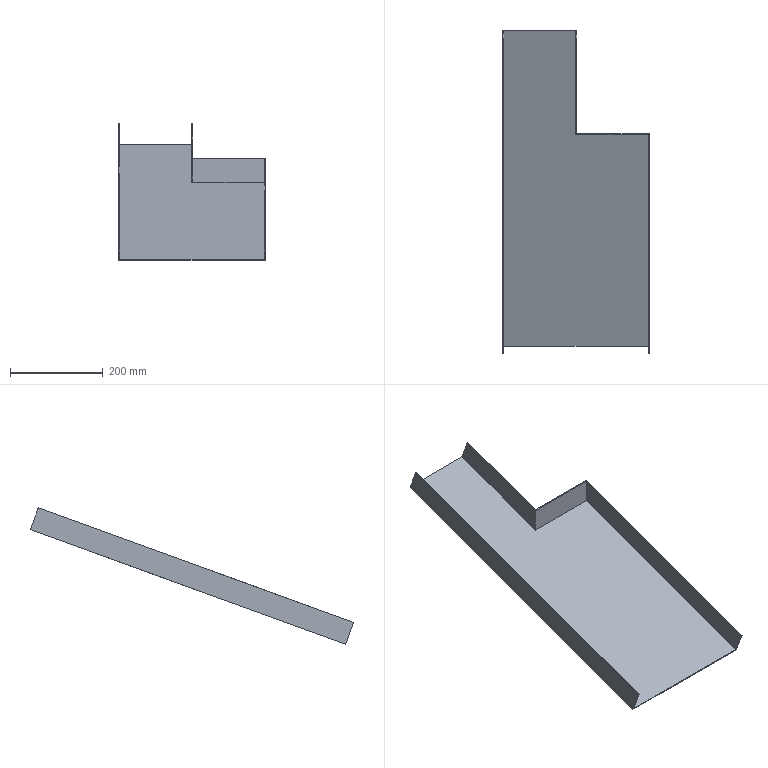Part | NX | features solid 2 | 1 solid | 14 faces | box 315 x 695.354 x 293.848 mm | volume 535547 mm3 | plane 14
STEP:
#1=CARTESIAN_POINT('',(-807.,-517.,-239.51));
#2=VERTEX_POINT('',#1);
#3=CARTESIAN_POINT('',(-963.,-517.,-239.51));
#4=VERTEX_POINT('',#3);
#5=CARTESIAN_POINT('',(-1225.,-517.,-239.51));
#6=DIRECTION('',(1.,0.,0.));
#7=VECTOR('',#6,1000.);
#8=LINE('',#5,#7);
#9=EDGE_CURVE('',#2,#4,#8,.F.);
#10=ORIENTED_EDGE('',*,*,#9,.T.);
#11=CARTESIAN_POINT('',(-963.,-293.385,-158.121));
#12=VERTEX_POINT('',#11);
#13=CARTESIAN_POINT('',(-963.,108.795,-11.739));
#14=DIRECTION('',(0.,0.9397,0.342));
#15=VECTOR('',#14,1000.);
#16=LINE('',#13,#15);
#17=EDGE_CURVE('',#4,#12,#16,.T.);
#18=ORIENTED_EDGE('',*,*,#17,.T.);
#19=CARTESIAN_POINT('',(-1118.,-293.385,-158.121));
#20=VERTEX_POINT('',#19);
#21=CARTESIAN_POINT('',(-1225.,-293.385,-158.121));
#22=DIRECTION('',(-1.,0.,0.));
#23=VECTOR('',#22,1000.);
#24=LINE('',#21,#23);
#25=EDGE_CURVE('',#20,#12,#24,.F.);
#26=ORIENTED_EDGE('',*,*,#25,.F.);
#27=CARTESIAN_POINT('',(-1118.,-971.638,-404.984));
#28=VERTEX_POINT('',#27);
#29=CARTESIAN_POINT('',(-1118.,108.795,-11.739));
#30=DIRECTION('',(0.,-0.9397,-0.342));
#31=VECTOR('',#30,1000.);
#32=LINE('',#29,#31);
#33=EDGE_CURVE('',#20,#28,#32,.T.);
#34=ORIENTED_EDGE('',*,*,#33,.T.);
#35=CARTESIAN_POINT('',(-807.,-971.638,-404.984));
#36=VERTEX_POINT('',#35);
#37=CARTESIAN_POINT('',(-1100.,-971.638,-404.984));
#38=DIRECTION('',(1.,0.,0.));
#39=VECTOR('',#38,1000.);
#40=LINE('',#37,#39);
#41=EDGE_CURVE('',#28,#36,#40,.T.);
#42=ORIENTED_EDGE('',*,*,#41,.T.);
#43=CARTESIAN_POINT('',(-807.,-515.684,-239.031));
#44=DIRECTION('',(0.,-0.9397,-0.342));
#45=VECTOR('',#44,1000.);
#46=LINE('',#43,#45);
#47=EDGE_CURVE('',#2,#36,#46,.T.);
#48=ORIENTED_EDGE('',*,*,#47,.F.);
#49=EDGE_LOOP('',(#10,#18,#26,#34,#42,#48));
#50=FACE_BOUND('',#49,.T.);
#51=CARTESIAN_POINT('',(-1225.,108.795,-11.739));
#52=DIRECTION('',(0.,0.342,-0.9397));
#53=DIRECTION('',(0.,-0.9397,-0.342));
#54=AXIS2_PLACEMENT_3D('',#51,#52,#53);
#55=PLANE('',#54);
#56=ADVANCED_FACE('',(#50),#55,.F.);
#57=CARTESIAN_POINT('',(-961.,-515.,-240.91));
#58=VERTEX_POINT('',#57);
#59=CARTESIAN_POINT('',(-961.,-515.,-187.701));
#60=VERTEX_POINT('',#59);
#61=CARTESIAN_POINT('',(-961.,-515.,-240.91));
#62=DIRECTION('',(0.,0.,-1.));
#63=VECTOR('',#62,1000.);
#64=LINE('',#61,#63);
#65=EDGE_CURVE('',#58,#60,#64,.F.);
#66=ORIENTED_EDGE('',*,*,#65,.F.);
#67=CARTESIAN_POINT('',(-961.,-292.701,-160.));
#68=VERTEX_POINT('',#67);
#69=CARTESIAN_POINT('',(-961.,109.479,-13.618));
#70=DIRECTION('',(0.,0.9397,0.342));
#71=VECTOR('',#70,1000.);
#72=LINE('',#69,#71);
#73=EDGE_CURVE('',#58,#68,#72,.T.);
#74=ORIENTED_EDGE('',*,*,#73,.T.);
#75=CARTESIAN_POINT('',(-961.,-309.802,-113.015));
#76=VERTEX_POINT('',#75);
#77=CARTESIAN_POINT('',(-961.,-292.701,-160.));
#78=DIRECTION('',(0.,-0.342,0.9397));
#79=VECTOR('',#78,1000.);
#80=LINE('',#77,#79);
#81=EDGE_CURVE('',#68,#76,#80,.T.);
#82=ORIENTED_EDGE('',*,*,#81,.T.);
#83=CARTESIAN_POINT('',(-961.,-532.101,-193.926));
#84=DIRECTION('',(0.,0.9397,0.342));
#85=VECTOR('',#84,1000.);
#86=LINE('',#83,#85);
#87=EDGE_CURVE('',#60,#76,#86,.T.);
#88=ORIENTED_EDGE('',*,*,#87,.F.);
#89=EDGE_LOOP('',(#66,#74,#82,#88));
#90=FACE_BOUND('',#89,.T.);
#91=CARTESIAN_POINT('',(-961.,109.479,-13.618));
#92=DIRECTION('',(-1.,0.,0.));
#93=DIRECTION('',(0.,0.,1.));
#94=AXIS2_PLACEMENT_3D('',#91,#92,#93);
#95=PLANE('',#94);
#96=ADVANCED_FACE('',(#90),#95,.F.);
#97=ORIENTED_EDGE('',*,*,#47,.T.);
#98=CARTESIAN_POINT('',(-807.,-988.055,-359.879));
#99=VERTEX_POINT('',#98);
#100=CARTESIAN_POINT('',(-807.,-988.055,-359.879));
#101=DIRECTION('',(0.,0.342,-0.9397));
#102=VECTOR('',#101,1000.);
#103=LINE('',#100,#102);
#104=EDGE_CURVE('',#99,#36,#103,.T.);
#105=ORIENTED_EDGE('',*,*,#104,.F.);
#106=CARTESIAN_POINT('',(-807.,-517.,-188.429));
#107=VERTEX_POINT('',#106);
#108=CARTESIAN_POINT('',(-807.,-532.101,-193.926));
#109=DIRECTION('',(0.,0.9397,0.342));
#110=VECTOR('',#109,1000.);
#111=LINE('',#108,#110);
#112=EDGE_CURVE('',#107,#99,#111,.F.);
#113=ORIENTED_EDGE('',*,*,#112,.F.);
#114=CARTESIAN_POINT('',(-807.,-517.,-240.91));
#115=DIRECTION('',(0.,0.,-1.));
#116=VECTOR('',#115,1000.);
#117=LINE('',#114,#116);
#118=EDGE_CURVE('',#2,#107,#117,.F.);
#119=ORIENTED_EDGE('',*,*,#118,.F.);
#120=EDGE_LOOP('',(#97,#105,#113,#119));
#121=FACE_BOUND('',#120,.T.);
#122=CARTESIAN_POINT('',(-807.,-532.101,-193.926));
#123=DIRECTION('',(-1.,0.,0.));
#124=DIRECTION('',(0.,0.,1.));
#125=AXIS2_PLACEMENT_3D('',#122,#123,#124);
#126=PLANE('',#125);
#127=ADVANCED_FACE('',(#121),#126,.T.);
#128=CARTESIAN_POINT('',(-1120.,-970.954,-406.864));
#129=VERTEX_POINT('',#128);
#130=CARTESIAN_POINT('',(-1120.,-988.055,-359.879));
#131=VERTEX_POINT('',#130);
#132=CARTESIAN_POINT('',(-1120.,-970.954,-406.864));
#133=DIRECTION('',(0.,-0.342,0.9397));
#134=VECTOR('',#133,1000.);
#135=LINE('',#132,#134);
#136=EDGE_CURVE('',#129,#131,#135,.T.);
#137=ORIENTED_EDGE('',*,*,#136,.F.);
#138=CARTESIAN_POINT('',(-805.,-970.954,-406.864));
#139=VERTEX_POINT('',#138);
#140=CARTESIAN_POINT('',(-1100.,-970.954,-406.864));
#141=DIRECTION('',(1.,0.,0.));
#142=VECTOR('',#141,1000.);
#143=LINE('',#140,#142);
#144=EDGE_CURVE('',#129,#139,#143,.T.);
#145=ORIENTED_EDGE('',*,*,#144,.T.);
#146=CARTESIAN_POINT('',(-805.,-988.055,-359.879));
#147=VERTEX_POINT('',#146);
#148=CARTESIAN_POINT('',(-805.,-970.954,-406.864));
#149=DIRECTION('',(0.,-0.342,0.9397));
#150=VECTOR('',#149,1000.);
#151=LINE('',#148,#150);
#152=EDGE_CURVE('',#139,#147,#151,.T.);
#153=ORIENTED_EDGE('',*,*,#152,.T.);
#154=CARTESIAN_POINT('',(-870.,-988.055,-359.879));
#155=DIRECTION('',(1.,0.,0.));
#156=VECTOR('',#155,1000.);
#157=LINE('',#154,#156);
#158=EDGE_CURVE('',#147,#99,#157,.F.);
#159=ORIENTED_EDGE('',*,*,#158,.T.);
#160=ORIENTED_EDGE('',*,*,#104,.T.);
#161=ORIENTED_EDGE('',*,*,#41,.F.);
#162=CARTESIAN_POINT('',(-1118.,-988.055,-359.879));
#163=VERTEX_POINT('',#162);
#164=CARTESIAN_POINT('',(-1118.,-988.055,-359.879));
#165=DIRECTION('',(0.,0.342,-0.9397));
#166=VECTOR('',#165,1000.);
#167=LINE('',#164,#166);
#168=EDGE_CURVE('',#163,#28,#167,.T.);
#169=ORIENTED_EDGE('',*,*,#168,.F.);
#170=CARTESIAN_POINT('',(-1120.,-988.055,-359.879));
#171=DIRECTION('',(1.,0.,0.));
#172=VECTOR('',#171,1000.);
#173=LINE('',#170,#172);
#174=EDGE_CURVE('',#131,#163,#173,.T.);
#175=ORIENTED_EDGE('',*,*,#174,.F.);
#176=EDGE_LOOP('',(#137,#145,#153,#159,#160,#161,#169,#175));
#177=FACE_BOUND('',#176,.T.);
#178=CARTESIAN_POINT('',(-1100.,-970.954,-406.864));
#179=DIRECTION('',(0.,0.9397,0.342));
#180=DIRECTION('',(0.,0.342,-0.9397));
#181=AXIS2_PLACEMENT_3D('',#178,#179,#180);
#182=PLANE('',#181);
#183=ADVANCED_FACE('',(#177),#182,.F.);
#184=CARTESIAN_POINT('',(-1120.,-292.701,-160.));
#185=VERTEX_POINT('',#184);
#186=CARTESIAN_POINT('',(-1120.,-309.802,-113.015));
#187=VERTEX_POINT('',#186);
#188=CARTESIAN_POINT('',(-1120.,-292.701,-160.));
#189=DIRECTION('',(0.,-0.342,0.9397));
#190=VECTOR('',#189,1000.);
#191=LINE('',#188,#190);
#192=EDGE_CURVE('',#185,#187,#191,.T.);
#193=ORIENTED_EDGE('',*,*,#192,.F.);
#194=CARTESIAN_POINT('',(-1120.,109.479,-13.618));
#195=DIRECTION('',(0.,0.9397,0.342));
#196=VECTOR('',#195,1000.);
#197=LINE('',#194,#196);
#198=EDGE_CURVE('',#185,#129,#197,.F.);
#199=ORIENTED_EDGE('',*,*,#198,.T.);
#200=ORIENTED_EDGE('',*,*,#136,.T.);
#201=CARTESIAN_POINT('',(-1120.,-309.802,-113.015));
#202=DIRECTION('',(0.,-0.9397,-0.342));
#203=VECTOR('',#202,1000.);
#204=LINE('',#201,#203);
#205=EDGE_CURVE('',#187,#131,#204,.T.);
#206=ORIENTED_EDGE('',*,*,#205,.F.);
#207=EDGE_LOOP('',(#193,#199,#200,#206));
#208=FACE_BOUND('',#207,.T.);
#209=CARTESIAN_POINT('',(-1120.,109.479,-13.618));
#210=DIRECTION('',(1.,0.,0.));
#211=DIRECTION('',(0.,0.,-1.));
#212=AXIS2_PLACEMENT_3D('',#209,#210,#211);
#213=PLANE('',#212);
#214=ADVANCED_FACE('',(#208),#213,.F.);
#215=CARTESIAN_POINT('',(-1225.,-292.701,-160.));
#216=DIRECTION('',(-1.,0.,0.));
#217=VECTOR('',#216,1000.);
#218=LINE('',#215,#217);
#219=EDGE_CURVE('',#185,#68,#218,.F.);
#220=ORIENTED_EDGE('',*,*,#219,.F.);
#221=ORIENTED_EDGE('',*,*,#192,.T.);
#222=CARTESIAN_POINT('',(-1118.,-309.802,-113.015));
#223=VERTEX_POINT('',#222);
#224=CARTESIAN_POINT('',(-1120.,-309.802,-113.015));
#225=DIRECTION('',(1.,0.,0.));
#226=VECTOR('',#225,1000.);
#227=LINE('',#224,#226);
#228=EDGE_CURVE('',#187,#223,#227,.T.);
#229=ORIENTED_EDGE('',*,*,#228,.T.);
#230=CARTESIAN_POINT('',(-1118.,-309.802,-113.015));
#231=DIRECTION('',(0.,0.342,-0.9397));
#232=VECTOR('',#231,1000.);
#233=LINE('',#230,#232);
#234=EDGE_CURVE('',#223,#20,#233,.T.);
#235=ORIENTED_EDGE('',*,*,#234,.T.);
#236=ORIENTED_EDGE('',*,*,#25,.T.);
#237=CARTESIAN_POINT('',(-963.,-309.802,-113.015));
#238=VERTEX_POINT('',#237);
#239=CARTESIAN_POINT('',(-963.,-309.802,-113.015));
#240=DIRECTION('',(0.,0.342,-0.9397));
#241=VECTOR('',#240,1000.);
#242=LINE('',#239,#241);
#243=EDGE_CURVE('',#238,#12,#242,.T.);
#244=ORIENTED_EDGE('',*,*,#243,.F.);
#245=CARTESIAN_POINT('',(-961.,-309.802,-113.015));
#246=DIRECTION('',(1.,0.,0.));
#247=VECTOR('',#246,1000.);
#248=LINE('',#245,#247);
#249=EDGE_CURVE('',#76,#238,#248,.F.);
#250=ORIENTED_EDGE('',*,*,#249,.F.);
#251=ORIENTED_EDGE('',*,*,#81,.F.);
#252=EDGE_LOOP('',(#220,#221,#229,#235,#236,#244,#250,#251));
#253=FACE_BOUND('',#252,.T.);
#254=CARTESIAN_POINT('',(-1225.,-292.701,-160.));
#255=DIRECTION('',(0.,0.9397,0.342));
#256=DIRECTION('',(0.,0.342,-0.9397));
#257=AXIS2_PLACEMENT_3D('',#254,#255,#256);
#258=PLANE('',#257);
#259=ADVANCED_FACE('',(#253),#258,.T.);
#260=CARTESIAN_POINT('',(-805.,-515.,-187.701));
#261=VERTEX_POINT('',#260);
#262=CARTESIAN_POINT('',(-805.,-532.101,-193.926));
#263=DIRECTION('',(0.,0.9397,0.342));
#264=VECTOR('',#263,1000.);
#265=LINE('',#262,#264);
#266=EDGE_CURVE('',#261,#147,#265,.F.);
#267=ORIENTED_EDGE('',*,*,#266,.T.);
#268=ORIENTED_EDGE('',*,*,#152,.F.);
#269=CARTESIAN_POINT('',(-805.,-515.,-240.91));
#270=VERTEX_POINT('',#269);
#271=CARTESIAN_POINT('',(-805.,109.479,-13.618));
#272=DIRECTION('',(0.,-0.9397,-0.342));
#273=VECTOR('',#272,1000.);
#274=LINE('',#271,#273);
#275=EDGE_CURVE('',#270,#139,#274,.T.);
#276=ORIENTED_EDGE('',*,*,#275,.F.);
#277=CARTESIAN_POINT('',(-805.,-515.,-240.91));
#278=DIRECTION('',(0.,0.,1.));
#279=VECTOR('',#278,1000.);
#280=LINE('',#277,#279);
#281=EDGE_CURVE('',#270,#261,#280,.T.);
#282=ORIENTED_EDGE('',*,*,#281,.T.);
#283=EDGE_LOOP('',(#267,#268,#276,#282));
#284=FACE_BOUND('',#283,.T.);
#285=CARTESIAN_POINT('',(-805.,109.479,-13.618));
#286=DIRECTION('',(1.,0.,0.));
#287=DIRECTION('',(0.,0.,-1.));
#288=AXIS2_PLACEMENT_3D('',#285,#286,#287);
#289=PLANE('',#288);
#290=ADVANCED_FACE('',(#284),#289,.T.);
#291=ORIENTED_EDGE('',*,*,#144,.F.);
#292=ORIENTED_EDGE('',*,*,#198,.F.);
#293=ORIENTED_EDGE('',*,*,#219,.T.);
#294=ORIENTED_EDGE('',*,*,#73,.F.);
#295=CARTESIAN_POINT('',(-1225.,-515.,-240.91));
#296=DIRECTION('',(-1.,0.,0.));
#297=VECTOR('',#296,1000.);
#298=LINE('',#295,#297);
#299=EDGE_CURVE('',#270,#58,#298,.T.);
#300=ORIENTED_EDGE('',*,*,#299,.F.);
#301=ORIENTED_EDGE('',*,*,#275,.T.);
#302=EDGE_LOOP('',(#291,#292,#293,#294,#300,#301));
#303=FACE_BOUND('',#302,.T.);
#304=CARTESIAN_POINT('',(-1225.,109.479,-13.618));
#305=DIRECTION('',(0.,0.342,-0.9397));
#306=DIRECTION('',(0.,-0.9397,-0.342));
#307=AXIS2_PLACEMENT_3D('',#304,#305,#306);
#308=PLANE('',#307);
#309=ADVANCED_FACE('',(#303),#308,.T.);
#310=CARTESIAN_POINT('',(-963.,-517.,-188.429));
#311=VERTEX_POINT('',#310);
#312=CARTESIAN_POINT('',(-961.,-517.,-188.429));
#313=DIRECTION('',(-1.,0.,0.));
#314=VECTOR('',#313,1000.);
#315=LINE('',#312,#314);
#316=EDGE_CURVE('',#107,#311,#315,.T.);
#317=ORIENTED_EDGE('',*,*,#316,.T.);
#318=CARTESIAN_POINT('',(-963.,-517.,-193.926));
#319=DIRECTION('',(0.,0.,1.));
#320=VECTOR('',#319,1000.);
#321=LINE('',#318,#320);
#322=EDGE_CURVE('',#311,#4,#321,.F.);
#323=ORIENTED_EDGE('',*,*,#322,.T.);
#324=ORIENTED_EDGE('',*,*,#9,.F.);
#325=ORIENTED_EDGE('',*,*,#118,.T.);
#326=EDGE_LOOP('',(#317,#323,#324,#325));
#327=FACE_BOUND('',#326,.T.);
#328=CARTESIAN_POINT('',(-870.,-517.,-240.91));
#329=DIRECTION('',(0.,-1.,0.));
#330=DIRECTION('',(-1.,0.,0.));
#331=AXIS2_PLACEMENT_3D('',#328,#329,#330);
#332=PLANE('',#331);
#333=ADVANCED_FACE('',(#327),#332,.T.);
#334=ORIENTED_EDGE('',*,*,#322,.F.);
#335=CARTESIAN_POINT('',(-963.,-532.101,-193.926));
#336=DIRECTION('',(0.,0.9397,0.342));
#337=VECTOR('',#336,1000.);
#338=LINE('',#335,#337);
#339=EDGE_CURVE('',#311,#238,#338,.T.);
#340=ORIENTED_EDGE('',*,*,#339,.T.);
#341=ORIENTED_EDGE('',*,*,#243,.T.);
#342=ORIENTED_EDGE('',*,*,#17,.F.);
#343=EDGE_LOOP('',(#334,#340,#341,#342));
#344=FACE_BOUND('',#343,.T.);
#345=CARTESIAN_POINT('',(-963.,-532.101,-193.926));
#346=DIRECTION('',(1.,0.,0.));
#347=DIRECTION('',(0.,0.,-1.));
#348=AXIS2_PLACEMENT_3D('',#345,#346,#347);
#349=PLANE('',#348);
#350=ADVANCED_FACE('',(#344),#349,.F.);
#351=ORIENTED_EDGE('',*,*,#316,.F.);
#352=ORIENTED_EDGE('',*,*,#112,.T.);
#353=ORIENTED_EDGE('',*,*,#158,.F.);
#354=ORIENTED_EDGE('',*,*,#266,.F.);
#355=CARTESIAN_POINT('',(-870.,-515.,-187.701));
#356=DIRECTION('',(-1.,0.,0.));
#357=VECTOR('',#356,1000.);
#358=LINE('',#355,#357);
#359=EDGE_CURVE('',#261,#60,#358,.T.);
#360=ORIENTED_EDGE('',*,*,#359,.T.);
#361=ORIENTED_EDGE('',*,*,#87,.T.);
#362=ORIENTED_EDGE('',*,*,#249,.T.);
#363=ORIENTED_EDGE('',*,*,#339,.F.);
#364=EDGE_LOOP('',(#351,#352,#353,#354,#360,#361,#362,#363));
#365=FACE_BOUND('',#364,.T.);
#366=CARTESIAN_POINT('',(-961.,-532.101,-193.926));
#367=DIRECTION('',(0.,-0.342,0.9397));
#368=DIRECTION('',(0.,0.9397,0.342));
#369=AXIS2_PLACEMENT_3D('',#366,#367,#368);
#370=PLANE('',#369);
#371=ADVANCED_FACE('',(#365),#370,.T.);
#372=ORIENTED_EDGE('',*,*,#234,.F.);
#373=CARTESIAN_POINT('',(-1118.,-309.802,-113.015));
#374=DIRECTION('',(0.,-0.9397,-0.342));
#375=VECTOR('',#374,1000.);
#376=LINE('',#373,#375);
#377=EDGE_CURVE('',#223,#163,#376,.T.);
#378=ORIENTED_EDGE('',*,*,#377,.T.);
#379=ORIENTED_EDGE('',*,*,#168,.T.);
#380=ORIENTED_EDGE('',*,*,#33,.F.);
#381=EDGE_LOOP('',(#372,#378,#379,#380));
#382=FACE_BOUND('',#381,.T.);
#383=CARTESIAN_POINT('',(-1118.,-309.802,-113.015));
#384=DIRECTION('',(-1.,0.,0.));
#385=DIRECTION('',(0.,0.,1.));
#386=AXIS2_PLACEMENT_3D('',#383,#384,#385);
#387=PLANE('',#386);
#388=ADVANCED_FACE('',(#382),#387,.F.);
#389=ORIENTED_EDGE('',*,*,#174,.T.);
#390=ORIENTED_EDGE('',*,*,#377,.F.);
#391=ORIENTED_EDGE('',*,*,#228,.F.);
#392=ORIENTED_EDGE('',*,*,#205,.T.);
#393=EDGE_LOOP('',(#389,#390,#391,#392));
#394=FACE_BOUND('',#393,.T.);
#395=CARTESIAN_POINT('',(-1120.,-309.802,-113.015));
#396=DIRECTION('',(0.,-0.342,0.9397));
#397=DIRECTION('',(0.,-0.9397,-0.342));
#398=AXIS2_PLACEMENT_3D('',#395,#396,#397);
#399=PLANE('',#398);
#400=ADVANCED_FACE('',(#394),#399,.T.);
#401=ORIENTED_EDGE('',*,*,#281,.F.);
#402=ORIENTED_EDGE('',*,*,#299,.T.);
#403=ORIENTED_EDGE('',*,*,#65,.T.);
#404=ORIENTED_EDGE('',*,*,#359,.F.);
#405=EDGE_LOOP('',(#401,#402,#403,#404));
#406=FACE_BOUND('',#405,.T.);
#407=CARTESIAN_POINT('',(-870.,-515.,-240.91));
#408=DIRECTION('',(0.,-1.,0.));
#409=DIRECTION('',(-1.,0.,0.));
#410=AXIS2_PLACEMENT_3D('',#407,#408,#409);
#411=PLANE('',#410);
#412=ADVANCED_FACE('',(#406),#411,.F.);
#413=CLOSED_SHELL('',(#56,#96,#127,#183,#214,#259,#290,#309,#333,#350,#371,#388,#400,#412));
#414=MANIFOLD_SOLID_BREP('',#413);
#415=(LENGTH_UNIT()NAMED_UNIT(*)SI_UNIT(.MILLI.,.METRE.));
#416=UNCERTAINTY_MEASURE_WITH_UNIT(LENGTH_MEASURE(0.00001),#415,'','');
#417=(NAMED_UNIT(*)PLANE_ANGLE_UNIT()SI_UNIT($,.RADIAN.));
#418=(NAMED_UNIT(*)SI_UNIT($,.STERADIAN.)SOLID_ANGLE_UNIT());
#419=(GEOMETRIC_REPRESENTATION_CONTEXT(3)GLOBAL_UNCERTAINTY_ASSIGNED_CONTEXT((#416))GLOBAL_UNIT_ASSIGNED_CONTEXT((#415,#417,#418))REPRESENTATION_CONTEXT('',''));
#420=ADVANCED_BREP_SHAPE_REPRESENTATION('',(#414),#419);